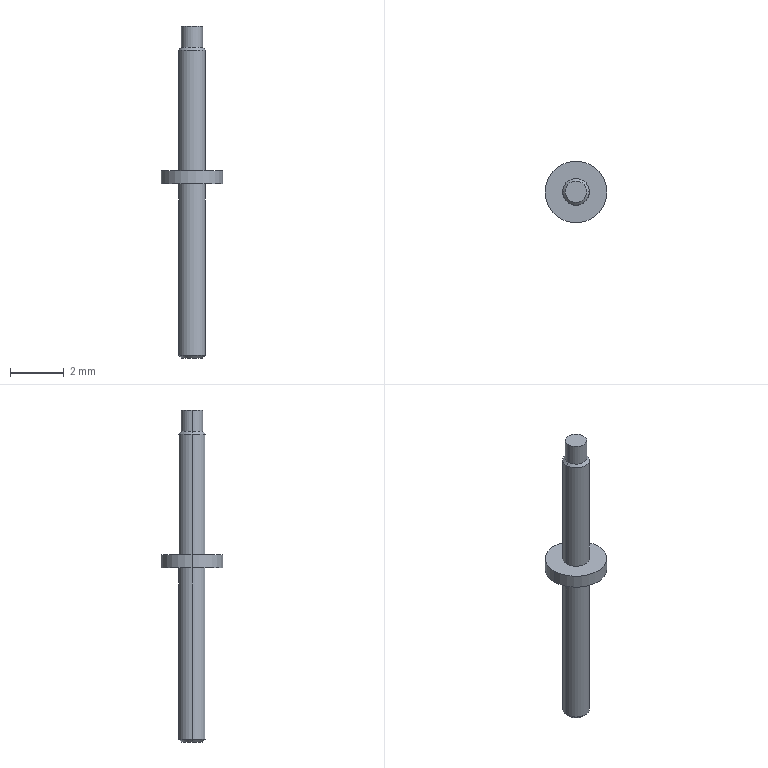Part | SolidWorks | features ICE 3, Chamfer 1, Extrusion 1 | 1 solid | 16 faces | box 2.3 x 2.3 x 12.4 mm | volume 11.168 mm3 | cylinder 8 | cone 4 | plane 4 | commonest cylinder face diameters 1 x4 0.8 x2 2.3 x2
STEP:
#1=CARTESIAN_POINT('',(-0.4,0.,-6.5));
#2=VERTEX_POINT('',#1);
#3=CARTESIAN_POINT('',(0.4,0.,-6.5));
#4=VERTEX_POINT('',#3);
#5=CARTESIAN_POINT('',(0.,0.,-6.5));
#6=DIRECTION('',(0.,0.,-1.));
#7=DIRECTION('',(-1.,0.,0.));
#8=AXIS2_PLACEMENT_3D('',#5,#6,#7);
#9=CIRCLE('',#8,0.4);
#10=EDGE_CURVE('',#2,#4,#9,.T.);
#11=ORIENTED_EDGE('',*,*,#10,.F.);
#12=CARTESIAN_POINT('',(-0.5,0.,-6.4));
#13=VERTEX_POINT('',#12);
#14=CARTESIAN_POINT('',(-0.4,0.,-6.5));
#15=DIRECTION('',(-0.7071,0.,0.7071));
#16=VECTOR('',#15,1000.);
#17=LINE('',#14,#16);
#18=EDGE_CURVE('',#2,#13,#17,.T.);
#19=ORIENTED_EDGE('',*,*,#18,.T.);
#20=CARTESIAN_POINT('',(0.5,0.,-6.4));
#21=VERTEX_POINT('',#20);
#22=CARTESIAN_POINT('',(0.,0.,-6.4));
#23=DIRECTION('',(0.,0.,1.));
#24=DIRECTION('',(-1.,0.,0.));
#25=AXIS2_PLACEMENT_3D('',#22,#23,#24);
#26=CIRCLE('',#25,0.5);
#27=EDGE_CURVE('',#21,#13,#26,.T.);
#28=ORIENTED_EDGE('',*,*,#27,.F.);
#29=CARTESIAN_POINT('',(0.4,0.,-6.5));
#30=DIRECTION('',(0.7071,0.,0.7071));
#31=VECTOR('',#30,1000.);
#32=LINE('',#29,#31);
#33=EDGE_CURVE('',#4,#21,#32,.T.);
#34=ORIENTED_EDGE('',*,*,#33,.F.);
#35=EDGE_LOOP('',(#11,#19,#28,#34));
#36=FACE_OUTER_BOUND('',#35,.T.);
#37=CARTESIAN_POINT('',(0.,0.,-6.5));
#38=DIRECTION('',(0.,0.,1.));
#39=DIRECTION('',(1.,0.,0.));
#40=AXIS2_PLACEMENT_3D('',#37,#38,#39);
#41=CONICAL_SURFACE('',#40,0.4,0.7854);
#42=ADVANCED_FACE('',(#36),#41,.T.);
#43=CARTESIAN_POINT('',(0.4,0.,5.1));
#44=VERTEX_POINT('',#43);
#45=CARTESIAN_POINT('',(-0.4,0.,5.1));
#46=VERTEX_POINT('',#45);
#47=CARTESIAN_POINT('',(0.,0.,5.1));
#48=DIRECTION('',(0.,0.,1.));
#49=DIRECTION('',(1.,0.,0.));
#50=AXIS2_PLACEMENT_3D('',#47,#48,#49);
#51=CIRCLE('',#50,0.4);
#52=EDGE_CURVE('',#44,#46,#51,.T.);
#53=ORIENTED_EDGE('',*,*,#52,.F.);
#54=CARTESIAN_POINT('',(0.5,0.,5.));
#55=VERTEX_POINT('',#54);
#56=CARTESIAN_POINT('',(0.4,0.,5.1));
#57=DIRECTION('',(0.7071,0.,-0.7071));
#58=VECTOR('',#57,1000.);
#59=LINE('',#56,#58);
#60=EDGE_CURVE('',#44,#55,#59,.T.);
#61=ORIENTED_EDGE('',*,*,#60,.T.);
#62=CARTESIAN_POINT('',(-0.5,0.,5.));
#63=VERTEX_POINT('',#62);
#64=CARTESIAN_POINT('',(0.,0.,5.));
#65=DIRECTION('',(0.,0.,-1.));
#66=DIRECTION('',(1.,0.,0.));
#67=AXIS2_PLACEMENT_3D('',#64,#65,#66);
#68=CIRCLE('',#67,0.5);
#69=EDGE_CURVE('',#63,#55,#68,.T.);
#70=ORIENTED_EDGE('',*,*,#69,.F.);
#71=CARTESIAN_POINT('',(-0.4,0.,5.1));
#72=DIRECTION('',(-0.7071,0.,-0.7071));
#73=VECTOR('',#72,1000.);
#74=LINE('',#71,#73);
#75=EDGE_CURVE('',#46,#63,#74,.T.);
#76=ORIENTED_EDGE('',*,*,#75,.F.);
#77=EDGE_LOOP('',(#53,#61,#70,#76));
#78=FACE_OUTER_BOUND('',#77,.T.);
#79=CARTESIAN_POINT('',(0.,0.,5.1));
#80=DIRECTION('',(0.,0.,-1.));
#81=DIRECTION('',(-1.,0.,0.));
#82=AXIS2_PLACEMENT_3D('',#79,#80,#81);
#83=CONICAL_SURFACE('',#82,0.4,0.7854);
#84=ADVANCED_FACE('',(#78),#83,.T.);
#85=ORIENTED_EDGE('',*,*,#27,.T.);
#86=CARTESIAN_POINT('',(-0.5,0.,0.));
#87=VERTEX_POINT('',#86);
#88=CARTESIAN_POINT('',(-0.5,0.,-6.5));
#89=DIRECTION('',(0.,0.,1.));
#90=VECTOR('',#89,1000.);
#91=LINE('',#88,#90);
#92=EDGE_CURVE('',#13,#87,#91,.T.);
#93=ORIENTED_EDGE('',*,*,#92,.T.);
#94=CARTESIAN_POINT('',(0.5,0.,0.));
#95=VERTEX_POINT('',#94);
#96=CARTESIAN_POINT('',(0.,0.,0.));
#97=DIRECTION('',(0.,0.,-1.));
#98=DIRECTION('',(1.,0.,0.));
#99=AXIS2_PLACEMENT_3D('',#96,#97,#98);
#100=CIRCLE('',#99,0.5);
#101=EDGE_CURVE('',#87,#95,#100,.T.);
#102=ORIENTED_EDGE('',*,*,#101,.T.);
#103=CARTESIAN_POINT('',(0.5,0.,-6.5));
#104=DIRECTION('',(0.,0.,1.));
#105=VECTOR('',#104,1000.);
#106=LINE('',#103,#105);
#107=EDGE_CURVE('',#21,#95,#106,.T.);
#108=ORIENTED_EDGE('',*,*,#107,.F.);
#109=EDGE_LOOP('',(#85,#93,#102,#108));
#110=FACE_OUTER_BOUND('',#109,.T.);
#111=CARTESIAN_POINT('',(0.,0.,-6.5));
#112=DIRECTION('',(0.,0.,1.));
#113=DIRECTION('',(1.,0.,0.));
#114=AXIS2_PLACEMENT_3D('',#111,#112,#113);
#115=CYLINDRICAL_SURFACE('',#114,0.5);
#116=ADVANCED_FACE('',(#110),#115,.T.);
#117=CARTESIAN_POINT('',(0.4,0.,5.9));
#118=VERTEX_POINT('',#117);
#119=CARTESIAN_POINT('',(-0.4,0.,5.9));
#120=VERTEX_POINT('',#119);
#121=CARTESIAN_POINT('',(0.,0.,5.9));
#122=DIRECTION('',(0.,0.,1.));
#123=DIRECTION('',(1.,0.,0.));
#124=AXIS2_PLACEMENT_3D('',#121,#122,#123);
#125=CIRCLE('',#124,0.4);
#126=EDGE_CURVE('',#118,#120,#125,.T.);
#127=ORIENTED_EDGE('',*,*,#126,.F.);
#128=CARTESIAN_POINT('',(0.4,0.,5.9));
#129=DIRECTION('',(0.,0.,-1.));
#130=VECTOR('',#129,1000.);
#131=LINE('',#128,#130);
#132=EDGE_CURVE('',#118,#44,#131,.T.);
#133=ORIENTED_EDGE('',*,*,#132,.T.);
#134=ORIENTED_EDGE('',*,*,#52,.T.);
#135=CARTESIAN_POINT('',(-0.4,0.,5.9));
#136=DIRECTION('',(0.,0.,-1.));
#137=VECTOR('',#136,1000.);
#138=LINE('',#135,#137);
#139=EDGE_CURVE('',#120,#46,#138,.T.);
#140=ORIENTED_EDGE('',*,*,#139,.F.);
#141=EDGE_LOOP('',(#127,#133,#134,#140));
#142=FACE_OUTER_BOUND('',#141,.T.);
#143=CARTESIAN_POINT('',(0.,0.,5.9));
#144=DIRECTION('',(0.,0.,-1.));
#145=DIRECTION('',(-1.,0.,0.));
#146=AXIS2_PLACEMENT_3D('',#143,#144,#145);
#147=CYLINDRICAL_SURFACE('',#146,0.4);
#148=ADVANCED_FACE('',(#142),#147,.T.);
#149=ORIENTED_EDGE('',*,*,#69,.T.);
#150=CARTESIAN_POINT('',(0.5,0.,0.5));
#151=VERTEX_POINT('',#150);
#152=CARTESIAN_POINT('',(0.5,0.,5.1));
#153=DIRECTION('',(0.,0.,-1.));
#154=VECTOR('',#153,1000.);
#155=LINE('',#152,#154);
#156=EDGE_CURVE('',#55,#151,#155,.T.);
#157=ORIENTED_EDGE('',*,*,#156,.T.);
#158=CARTESIAN_POINT('',(-0.5,0.,0.5));
#159=VERTEX_POINT('',#158);
#160=CARTESIAN_POINT('',(0.,0.,0.5));
#161=DIRECTION('',(0.,0.,1.));
#162=DIRECTION('',(1.,0.,0.));
#163=AXIS2_PLACEMENT_3D('',#160,#161,#162);
#164=CIRCLE('',#163,0.5);
#165=EDGE_CURVE('',#151,#159,#164,.T.);
#166=ORIENTED_EDGE('',*,*,#165,.T.);
#167=CARTESIAN_POINT('',(-0.5,0.,5.1));
#168=DIRECTION('',(0.,0.,-1.));
#169=VECTOR('',#168,1000.);
#170=LINE('',#167,#169);
#171=EDGE_CURVE('',#63,#159,#170,.T.);
#172=ORIENTED_EDGE('',*,*,#171,.F.);
#173=EDGE_LOOP('',(#149,#157,#166,#172));
#174=FACE_OUTER_BOUND('',#173,.T.);
#175=CARTESIAN_POINT('',(0.,0.,5.1));
#176=DIRECTION('',(0.,0.,-1.));
#177=DIRECTION('',(-1.,0.,0.));
#178=AXIS2_PLACEMENT_3D('',#175,#176,#177);
#179=CYLINDRICAL_SURFACE('',#178,0.5);
#180=ADVANCED_FACE('',(#174),#179,.T.);
#181=CARTESIAN_POINT('',(1.15,0.,0.5));
#182=VERTEX_POINT('',#181);
#183=CARTESIAN_POINT('',(-1.15,0.,0.5));
#184=VERTEX_POINT('',#183);
#185=CARTESIAN_POINT('',(0.,0.,0.5));
#186=DIRECTION('',(0.,0.,1.));
#187=DIRECTION('',(1.,0.,0.));
#188=AXIS2_PLACEMENT_3D('',#185,#186,#187);
#189=CIRCLE('',#188,1.15);
#190=EDGE_CURVE('',#182,#184,#189,.T.);
#191=ORIENTED_EDGE('',*,*,#190,.F.);
#192=CARTESIAN_POINT('',(1.15,0.,0.));
#193=VERTEX_POINT('',#192);
#194=CARTESIAN_POINT('',(1.15,0.,0.5));
#195=DIRECTION('',(0.,0.,-1.));
#196=VECTOR('',#195,1000.);
#197=LINE('',#194,#196);
#198=EDGE_CURVE('',#182,#193,#197,.T.);
#199=ORIENTED_EDGE('',*,*,#198,.T.);
#200=CARTESIAN_POINT('',(-1.15,0.,0.));
#201=VERTEX_POINT('',#200);
#202=CARTESIAN_POINT('',(0.,0.,0.));
#203=DIRECTION('',(0.,0.,1.));
#204=DIRECTION('',(1.,0.,0.));
#205=AXIS2_PLACEMENT_3D('',#202,#203,#204);
#206=CIRCLE('',#205,1.15);
#207=EDGE_CURVE('',#193,#201,#206,.T.);
#208=ORIENTED_EDGE('',*,*,#207,.T.);
#209=CARTESIAN_POINT('',(-1.15,0.,0.5));
#210=DIRECTION('',(0.,0.,-1.));
#211=VECTOR('',#210,1000.);
#212=LINE('',#209,#211);
#213=EDGE_CURVE('',#184,#201,#212,.T.);
#214=ORIENTED_EDGE('',*,*,#213,.F.);
#215=EDGE_LOOP('',(#191,#199,#208,#214));
#216=FACE_OUTER_BOUND('',#215,.T.);
#217=CARTESIAN_POINT('',(0.,0.,0.5));
#218=DIRECTION('',(0.,0.,-1.));
#219=DIRECTION('',(-1.,0.,0.));
#220=AXIS2_PLACEMENT_3D('',#217,#218,#219);
#221=CYLINDRICAL_SURFACE('',#220,1.15);
#222=ADVANCED_FACE('',(#216),#221,.T.);
#223=CARTESIAN_POINT('',(0.,0.,0.));
#224=DIRECTION('',(0.,0.,1.));
#225=DIRECTION('',(1.,0.,0.));
#226=AXIS2_PLACEMENT_3D('',#223,#224,#225);
#227=CIRCLE('',#226,1.15);
#228=EDGE_CURVE('',#201,#193,#227,.T.);
#229=ORIENTED_EDGE('',*,*,#228,.F.);
#230=ORIENTED_EDGE('',*,*,#207,.F.);
#231=EDGE_LOOP('',(#229,#230));
#232=FACE_OUTER_BOUND('',#231,.T.);
#233=CARTESIAN_POINT('',(0.,0.,0.));
#234=DIRECTION('',(0.,0.,-1.));
#235=DIRECTION('',(1.,0.,0.));
#236=AXIS2_PLACEMENT_3D('',#233,#234,#235);
#237=CIRCLE('',#236,0.5);
#238=EDGE_CURVE('',#95,#87,#237,.T.);
#239=ORIENTED_EDGE('',*,*,#238,.F.);
#240=ORIENTED_EDGE('',*,*,#101,.F.);
#241=EDGE_LOOP('',(#239,#240));
#242=FACE_BOUND('',#241,.T.);
#243=CARTESIAN_POINT('',(0.,0.,0.));
#244=DIRECTION('',(0.,0.,1.));
#245=DIRECTION('',(1.,0.,0.));
#246=AXIS2_PLACEMENT_3D('',#243,#244,#245);
#247=PLANE('',#246);
#248=ADVANCED_FACE('',(#232,#242),#247,.F.);
#249=CARTESIAN_POINT('',(0.,0.,0.5));
#250=DIRECTION('',(0.,0.,1.));
#251=DIRECTION('',(1.,0.,0.));
#252=AXIS2_PLACEMENT_3D('',#249,#250,#251);
#253=CIRCLE('',#252,1.15);
#254=EDGE_CURVE('',#184,#182,#253,.T.);
#255=ORIENTED_EDGE('',*,*,#254,.T.);
#256=ORIENTED_EDGE('',*,*,#190,.T.);
#257=EDGE_LOOP('',(#255,#256));
#258=FACE_OUTER_BOUND('',#257,.T.);
#259=CARTESIAN_POINT('',(0.,0.,0.5));
#260=DIRECTION('',(0.,0.,1.));
#261=DIRECTION('',(1.,0.,0.));
#262=AXIS2_PLACEMENT_3D('',#259,#260,#261);
#263=CIRCLE('',#262,0.5);
#264=EDGE_CURVE('',#159,#151,#263,.T.);
#265=ORIENTED_EDGE('',*,*,#264,.F.);
#266=ORIENTED_EDGE('',*,*,#165,.F.);
#267=EDGE_LOOP('',(#265,#266));
#268=FACE_BOUND('',#267,.T.);
#269=CARTESIAN_POINT('',(0.,0.,0.5));
#270=DIRECTION('',(0.,0.,1.));
#271=DIRECTION('',(1.,0.,0.));
#272=AXIS2_PLACEMENT_3D('',#269,#270,#271);
#273=PLANE('',#272);
#274=ADVANCED_FACE('',(#258,#268),#273,.T.);
#275=ORIENTED_EDGE('',*,*,#198,.F.);
#276=ORIENTED_EDGE('',*,*,#254,.F.);
#277=ORIENTED_EDGE('',*,*,#213,.T.);
#278=ORIENTED_EDGE('',*,*,#228,.T.);
#279=EDGE_LOOP('',(#275,#276,#277,#278));
#280=FACE_OUTER_BOUND('',#279,.T.);
#281=CARTESIAN_POINT('',(0.,0.,0.5));
#282=DIRECTION('',(0.,0.,-1.));
#283=DIRECTION('',(-1.,0.,0.));
#284=AXIS2_PLACEMENT_3D('',#281,#282,#283);
#285=CYLINDRICAL_SURFACE('',#284,1.15);
#286=ADVANCED_FACE('',(#280),#285,.T.);
#287=ORIENTED_EDGE('',*,*,#156,.F.);
#288=CARTESIAN_POINT('',(0.,0.,5.));
#289=DIRECTION('',(0.,0.,-1.));
#290=DIRECTION('',(1.,0.,0.));
#291=AXIS2_PLACEMENT_3D('',#288,#289,#290);
#292=CIRCLE('',#291,0.5);
#293=EDGE_CURVE('',#55,#63,#292,.T.);
#294=ORIENTED_EDGE('',*,*,#293,.T.);
#295=ORIENTED_EDGE('',*,*,#171,.T.);
#296=ORIENTED_EDGE('',*,*,#264,.T.);
#297=EDGE_LOOP('',(#287,#294,#295,#296));
#298=FACE_OUTER_BOUND('',#297,.T.);
#299=CARTESIAN_POINT('',(0.,0.,5.1));
#300=DIRECTION('',(0.,0.,-1.));
#301=DIRECTION('',(-1.,0.,0.));
#302=AXIS2_PLACEMENT_3D('',#299,#300,#301);
#303=CYLINDRICAL_SURFACE('',#302,0.5);
#304=ADVANCED_FACE('',(#298),#303,.T.);
#305=ORIENTED_EDGE('',*,*,#132,.F.);
#306=CARTESIAN_POINT('',(0.,0.,5.9));
#307=DIRECTION('',(0.,0.,1.));
#308=DIRECTION('',(1.,0.,0.));
#309=AXIS2_PLACEMENT_3D('',#306,#307,#308);
#310=CIRCLE('',#309,0.4);
#311=EDGE_CURVE('',#120,#118,#310,.T.);
#312=ORIENTED_EDGE('',*,*,#311,.F.);
#313=ORIENTED_EDGE('',*,*,#139,.T.);
#314=CARTESIAN_POINT('',(0.,0.,5.1));
#315=DIRECTION('',(0.,0.,1.));
#316=DIRECTION('',(1.,0.,0.));
#317=AXIS2_PLACEMENT_3D('',#314,#315,#316);
#318=CIRCLE('',#317,0.4);
#319=EDGE_CURVE('',#46,#44,#318,.T.);
#320=ORIENTED_EDGE('',*,*,#319,.T.);
#321=EDGE_LOOP('',(#305,#312,#313,#320));
#322=FACE_OUTER_BOUND('',#321,.T.);
#323=CARTESIAN_POINT('',(0.,0.,5.9));
#324=DIRECTION('',(0.,0.,-1.));
#325=DIRECTION('',(-1.,0.,0.));
#326=AXIS2_PLACEMENT_3D('',#323,#324,#325);
#327=CYLINDRICAL_SURFACE('',#326,0.4);
#328=ADVANCED_FACE('',(#322),#327,.T.);
#329=ORIENTED_EDGE('',*,*,#311,.T.);
#330=ORIENTED_EDGE('',*,*,#126,.T.);
#331=EDGE_LOOP('',(#329,#330));
#332=FACE_OUTER_BOUND('',#331,.T.);
#333=CARTESIAN_POINT('',(0.,0.,5.9));
#334=DIRECTION('',(0.,0.,1.));
#335=DIRECTION('',(1.,0.,0.));
#336=AXIS2_PLACEMENT_3D('',#333,#334,#335);
#337=PLANE('',#336);
#338=ADVANCED_FACE('',(#332),#337,.T.);
#339=ORIENTED_EDGE('',*,*,#92,.F.);
#340=CARTESIAN_POINT('',(0.,0.,-6.4));
#341=DIRECTION('',(0.,0.,1.));
#342=DIRECTION('',(-1.,0.,0.));
#343=AXIS2_PLACEMENT_3D('',#340,#341,#342);
#344=CIRCLE('',#343,0.5);
#345=EDGE_CURVE('',#13,#21,#344,.T.);
#346=ORIENTED_EDGE('',*,*,#345,.T.);
#347=ORIENTED_EDGE('',*,*,#107,.T.);
#348=ORIENTED_EDGE('',*,*,#238,.T.);
#349=EDGE_LOOP('',(#339,#346,#347,#348));
#350=FACE_OUTER_BOUND('',#349,.T.);
#351=CARTESIAN_POINT('',(0.,0.,-6.5));
#352=DIRECTION('',(0.,0.,1.));
#353=DIRECTION('',(1.,0.,0.));
#354=AXIS2_PLACEMENT_3D('',#351,#352,#353);
#355=CYLINDRICAL_SURFACE('',#354,0.5);
#356=ADVANCED_FACE('',(#350),#355,.T.);
#357=CARTESIAN_POINT('',(0.,0.,-6.5));
#358=DIRECTION('',(0.,0.,-1.));
#359=DIRECTION('',(-1.,0.,0.));
#360=AXIS2_PLACEMENT_3D('',#357,#358,#359);
#361=CIRCLE('',#360,0.4);
#362=EDGE_CURVE('',#4,#2,#361,.T.);
#363=ORIENTED_EDGE('',*,*,#362,.T.);
#364=ORIENTED_EDGE('',*,*,#10,.T.);
#365=EDGE_LOOP('',(#363,#364));
#366=FACE_OUTER_BOUND('',#365,.T.);
#367=CARTESIAN_POINT('',(0.,0.,-6.5));
#368=DIRECTION('',(0.,0.,-1.));
#369=DIRECTION('',(-1.,0.,0.));
#370=AXIS2_PLACEMENT_3D('',#367,#368,#369);
#371=PLANE('',#370);
#372=ADVANCED_FACE('',(#366),#371,.T.);
#373=ORIENTED_EDGE('',*,*,#60,.F.);
#374=ORIENTED_EDGE('',*,*,#319,.F.);
#375=ORIENTED_EDGE('',*,*,#75,.T.);
#376=ORIENTED_EDGE('',*,*,#293,.F.);
#377=EDGE_LOOP('',(#373,#374,#375,#376));
#378=FACE_OUTER_BOUND('',#377,.T.);
#379=CARTESIAN_POINT('',(0.,0.,5.1));
#380=DIRECTION('',(0.,0.,-1.));
#381=DIRECTION('',(-1.,0.,0.));
#382=AXIS2_PLACEMENT_3D('',#379,#380,#381);
#383=CONICAL_SURFACE('',#382,0.4,0.7854);
#384=ADVANCED_FACE('',(#378),#383,.T.);
#385=ORIENTED_EDGE('',*,*,#18,.F.);
#386=ORIENTED_EDGE('',*,*,#362,.F.);
#387=ORIENTED_EDGE('',*,*,#33,.T.);
#388=ORIENTED_EDGE('',*,*,#345,.F.);
#389=EDGE_LOOP('',(#385,#386,#387,#388));
#390=FACE_OUTER_BOUND('',#389,.T.);
#391=CARTESIAN_POINT('',(0.,0.,-6.5));
#392=DIRECTION('',(0.,0.,1.));
#393=DIRECTION('',(1.,0.,0.));
#394=AXIS2_PLACEMENT_3D('',#391,#392,#393);
#395=CONICAL_SURFACE('',#394,0.4,0.7854);
#396=ADVANCED_FACE('',(#390),#395,.T.);
#397=CLOSED_SHELL('',(#42,#84,#116,#148,#180,#222,#248,#274,#286,#304,#328,#338,#356,#372,#384,#396));
#398=MANIFOLD_SOLID_BREP('',#397);
#399=CARTESIAN_POINT('',(0.,0.,0.));
#400=DIRECTION('',(0.,0.,1.));
#401=DIRECTION('',(1.,0.,0.));
#402=AXIS2_PLACEMENT_3D('',#399,#400,#401);
#403=(LENGTH_UNIT()NAMED_UNIT(*)SI_UNIT(.MILLI.,.METRE.));
#404=UNCERTAINTY_MEASURE_WITH_UNIT(LENGTH_MEASURE(0.00001),#403,'','');
#405=(NAMED_UNIT(*)PLANE_ANGLE_UNIT()SI_UNIT($,.RADIAN.));
#406=(NAMED_UNIT(*)SI_UNIT($,.STERADIAN.)SOLID_ANGLE_UNIT());
#407=(GEOMETRIC_REPRESENTATION_CONTEXT(3)GLOBAL_UNCERTAINTY_ASSIGNED_CONTEXT((#404))GLOBAL_UNIT_ASSIGNED_CONTEXT((#403,#405,#406))REPRESENTATION_CONTEXT('',''));
#408=ADVANCED_BREP_SHAPE_REPRESENTATION('',(#398,#402),#407);